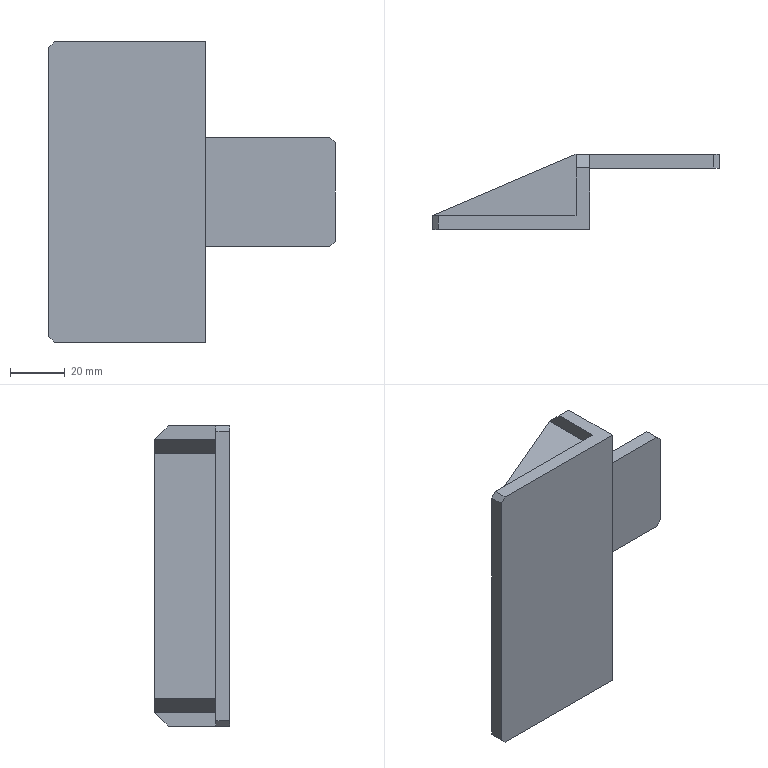Part | STEP file | Guide wheel mechanism revised.sldasm-Part-403 | 1 solid | 28 faces | box 105 x 27.5 x 110 mm | volume 59241 mm3 | plane 28
STEP:
#1=CARTESIAN_POINT('',(0.,22.5,45.));
#2=VERTEX_POINT('',#1);
#3=CARTESIAN_POINT('',(0.,22.5,-45.));
#4=VERTEX_POINT('',#3);
#5=CARTESIAN_POINT('',(0.,22.5,55.));
#6=DIRECTION('',(0.,0.,-1.));
#7=VECTOR('',#6,1000.);
#8=LINE('',#5,#7);
#9=EDGE_CURVE('',#2,#4,#8,.T.);
#10=ORIENTED_EDGE('',*,*,#9,.T.);
#11=CARTESIAN_POINT('',(0.,0.,-45.));
#12=VERTEX_POINT('',#11);
#13=CARTESIAN_POINT('',(0.,22.5,-45.));
#14=DIRECTION('',(0.,-1.,0.));
#15=VECTOR('',#14,1000.);
#16=LINE('',#13,#15);
#17=EDGE_CURVE('',#4,#12,#16,.T.);
#18=ORIENTED_EDGE('',*,*,#17,.T.);
#19=CARTESIAN_POINT('',(0.,0.,45.));
#20=VERTEX_POINT('',#19);
#21=CARTESIAN_POINT('',(0.,0.,55.));
#22=DIRECTION('',(0.,0.,-1.));
#23=VECTOR('',#22,1000.);
#24=LINE('',#21,#23);
#25=EDGE_CURVE('',#20,#12,#24,.T.);
#26=ORIENTED_EDGE('',*,*,#25,.F.);
#27=CARTESIAN_POINT('',(0.,22.5,45.));
#28=DIRECTION('',(0.,1.,0.));
#29=VECTOR('',#28,1000.);
#30=LINE('',#27,#29);
#31=EDGE_CURVE('',#20,#2,#30,.T.);
#32=ORIENTED_EDGE('',*,*,#31,.T.);
#33=EDGE_LOOP('',(#10,#18,#26,#32));
#34=FACE_OUTER_BOUND('',#33,.T.);
#35=CARTESIAN_POINT('',(0.,0.,55.));
#36=DIRECTION('',(-1.,0.,0.));
#37=DIRECTION('',(0.,0.,1.));
#38=AXIS2_PLACEMENT_3D('',#35,#36,#37);
#39=PLANE('',#38);
#40=ADVANCED_FACE('',(#34),#39,.T.);
#41=ORIENTED_EDGE('',*,*,#25,.T.);
#42=CARTESIAN_POINT('',(-52.5,0.,-45.));
#43=VERTEX_POINT('',#42);
#44=CARTESIAN_POINT('',(0.,0.,-45.));
#45=DIRECTION('',(-1.,0.,0.));
#46=VECTOR('',#45,1000.);
#47=LINE('',#44,#46);
#48=EDGE_CURVE('',#12,#43,#47,.T.);
#49=ORIENTED_EDGE('',*,*,#48,.T.);
#50=CARTESIAN_POINT('',(-52.5,0.,45.));
#51=VERTEX_POINT('',#50);
#52=CARTESIAN_POINT('',(-52.5,0.,55.));
#53=DIRECTION('',(0.,0.,-1.));
#54=VECTOR('',#53,1000.);
#55=LINE('',#52,#54);
#56=EDGE_CURVE('',#51,#43,#55,.T.);
#57=ORIENTED_EDGE('',*,*,#56,.F.);
#58=CARTESIAN_POINT('',(0.,0.,45.));
#59=DIRECTION('',(1.,0.,0.));
#60=VECTOR('',#59,1000.);
#61=LINE('',#58,#60);
#62=EDGE_CURVE('',#51,#20,#61,.T.);
#63=ORIENTED_EDGE('',*,*,#62,.T.);
#64=EDGE_LOOP('',(#41,#49,#57,#63));
#65=FACE_OUTER_BOUND('',#64,.T.);
#66=CARTESIAN_POINT('',(0.,0.,55.));
#67=DIRECTION('',(0.,1.,0.));
#68=DIRECTION('',(0.,0.,1.));
#69=AXIS2_PLACEMENT_3D('',#66,#67,#68);
#70=PLANE('',#69);
#71=ADVANCED_FACE('',(#65),#70,.T.);
#72=CARTESIAN_POINT('',(0.,22.5,-50.));
#73=VERTEX_POINT('',#72);
#74=CARTESIAN_POINT('',(0.,0.,-50.));
#75=VERTEX_POINT('',#74);
#76=CARTESIAN_POINT('',(0.,22.5,-50.));
#77=DIRECTION('',(0.,-1.,0.));
#78=VECTOR('',#77,1000.);
#79=LINE('',#76,#78);
#80=EDGE_CURVE('',#73,#75,#79,.T.);
#81=ORIENTED_EDGE('',*,*,#80,.F.);
#82=CARTESIAN_POINT('',(0.,17.5,-55.));
#83=VERTEX_POINT('',#82);
#84=CARTESIAN_POINT('',(0.,63.75,-8.75));
#85=DIRECTION('',(0.,-0.7071,-0.7071));
#86=VECTOR('',#85,1000.);
#87=LINE('',#84,#86);
#88=EDGE_CURVE('',#73,#83,#87,.T.);
#89=ORIENTED_EDGE('',*,*,#88,.T.);
#90=CARTESIAN_POINT('',(0.,0.,-55.));
#91=VERTEX_POINT('',#90);
#92=CARTESIAN_POINT('',(0.,0.,-55.));
#93=DIRECTION('',(0.,1.,0.));
#94=VECTOR('',#93,1000.);
#95=LINE('',#92,#94);
#96=EDGE_CURVE('',#91,#83,#95,.T.);
#97=ORIENTED_EDGE('',*,*,#96,.F.);
#98=CARTESIAN_POINT('',(0.,0.,55.));
#99=DIRECTION('',(0.,0.,-1.));
#100=VECTOR('',#99,1000.);
#101=LINE('',#98,#100);
#102=EDGE_CURVE('',#75,#91,#101,.T.);
#103=ORIENTED_EDGE('',*,*,#102,.F.);
#104=EDGE_LOOP('',(#81,#89,#97,#103));
#105=FACE_OUTER_BOUND('',#104,.T.);
#106=CARTESIAN_POINT('',(0.,0.,55.));
#107=DIRECTION('',(-1.,0.,0.));
#108=DIRECTION('',(0.,0.,1.));
#109=AXIS2_PLACEMENT_3D('',#106,#107,#108);
#110=PLANE('',#109);
#111=ADVANCED_FACE('',(#105),#110,.T.);
#112=CARTESIAN_POINT('',(-52.5,0.,-50.));
#113=VERTEX_POINT('',#112);
#114=CARTESIAN_POINT('',(0.,0.,-50.));
#115=DIRECTION('',(-1.,0.,0.));
#116=VECTOR('',#115,1000.);
#117=LINE('',#114,#116);
#118=EDGE_CURVE('',#75,#113,#117,.T.);
#119=ORIENTED_EDGE('',*,*,#118,.F.);
#120=ORIENTED_EDGE('',*,*,#102,.T.);
#121=CARTESIAN_POINT('',(-50.5,0.,-55.));
#122=VERTEX_POINT('',#121);
#123=CARTESIAN_POINT('',(0.,0.,-55.));
#124=DIRECTION('',(1.,0.,0.));
#125=VECTOR('',#124,1000.);
#126=LINE('',#123,#125);
#127=EDGE_CURVE('',#122,#91,#126,.T.);
#128=ORIENTED_EDGE('',*,*,#127,.F.);
#129=CARTESIAN_POINT('',(-52.5,0.,-53.));
#130=VERTEX_POINT('',#129);
#131=CARTESIAN_POINT('',(-80.25,0.,-25.25));
#132=DIRECTION('',(-0.7071,0.,0.7071));
#133=VECTOR('',#132,1000.);
#134=LINE('',#131,#133);
#135=EDGE_CURVE('',#122,#130,#134,.T.);
#136=ORIENTED_EDGE('',*,*,#135,.T.);
#137=CARTESIAN_POINT('',(-52.5,0.,55.));
#138=DIRECTION('',(0.,0.,-1.));
#139=VECTOR('',#138,1000.);
#140=LINE('',#137,#139);
#141=EDGE_CURVE('',#113,#130,#140,.T.);
#142=ORIENTED_EDGE('',*,*,#141,.F.);
#143=EDGE_LOOP('',(#119,#120,#128,#136,#142));
#144=FACE_OUTER_BOUND('',#143,.T.);
#145=CARTESIAN_POINT('',(0.,0.,55.));
#146=DIRECTION('',(0.,1.,0.));
#147=DIRECTION('',(0.,0.,1.));
#148=AXIS2_PLACEMENT_3D('',#145,#146,#147);
#149=PLANE('',#148);
#150=ADVANCED_FACE('',(#144),#149,.T.);
#151=CARTESIAN_POINT('',(50.5,17.5,-20.));
#152=VERTEX_POINT('',#151);
#153=CARTESIAN_POINT('',(5.,17.5,-20.));
#154=VERTEX_POINT('',#153);
#155=CARTESIAN_POINT('',(52.5,17.5,-20.));
#156=DIRECTION('',(-1.,0.,0.));
#157=VECTOR('',#156,1000.);
#158=LINE('',#155,#157);
#159=EDGE_CURVE('',#152,#154,#158,.T.);
#160=ORIENTED_EDGE('',*,*,#159,.F.);
#161=CARTESIAN_POINT('',(52.5,17.5,-18.));
#162=VERTEX_POINT('',#161);
#163=CARTESIAN_POINT('',(52.5,17.5,-18.));
#164=DIRECTION('',(0.7071,0.,0.7071));
#165=VECTOR('',#164,1000.);
#166=LINE('',#163,#165);
#167=EDGE_CURVE('',#152,#162,#166,.T.);
#168=ORIENTED_EDGE('',*,*,#167,.T.);
#169=CARTESIAN_POINT('',(52.5,17.5,18.));
#170=VERTEX_POINT('',#169);
#171=CARTESIAN_POINT('',(52.5,17.5,55.));
#172=DIRECTION('',(0.,0.,-1.));
#173=VECTOR('',#172,1000.);
#174=LINE('',#171,#173);
#175=EDGE_CURVE('',#170,#162,#174,.T.);
#176=ORIENTED_EDGE('',*,*,#175,.F.);
#177=CARTESIAN_POINT('',(50.5,17.5,20.));
#178=VERTEX_POINT('',#177);
#179=CARTESIAN_POINT('',(50.5,17.5,20.));
#180=DIRECTION('',(-0.7071,0.,0.7071));
#181=VECTOR('',#180,1000.);
#182=LINE('',#179,#181);
#183=EDGE_CURVE('',#170,#178,#182,.T.);
#184=ORIENTED_EDGE('',*,*,#183,.T.);
#185=CARTESIAN_POINT('',(5.,17.5,20.));
#186=VERTEX_POINT('',#185);
#187=CARTESIAN_POINT('',(52.5,17.5,20.));
#188=DIRECTION('',(1.,0.,0.));
#189=VECTOR('',#188,1000.);
#190=LINE('',#187,#189);
#191=EDGE_CURVE('',#186,#178,#190,.T.);
#192=ORIENTED_EDGE('',*,*,#191,.F.);
#193=CARTESIAN_POINT('',(5.,17.5,55.));
#194=DIRECTION('',(0.,0.,-1.));
#195=VECTOR('',#194,1000.);
#196=LINE('',#193,#195);
#197=EDGE_CURVE('',#186,#154,#196,.T.);
#198=ORIENTED_EDGE('',*,*,#197,.T.);
#199=EDGE_LOOP('',(#160,#168,#176,#184,#192,#198));
#200=FACE_OUTER_BOUND('',#199,.T.);
#201=CARTESIAN_POINT('',(0.,17.5,55.));
#202=DIRECTION('',(0.,1.,0.));
#203=DIRECTION('',(0.,0.,1.));
#204=AXIS2_PLACEMENT_3D('',#201,#202,#203);
#205=PLANE('',#204);
#206=ADVANCED_FACE('',(#200),#205,.F.);
#207=ORIENTED_EDGE('',*,*,#175,.T.);
#208=CARTESIAN_POINT('',(52.5,22.5,-18.));
#209=VERTEX_POINT('',#208);
#210=CARTESIAN_POINT('',(52.5,22.5,-18.));
#211=DIRECTION('',(0.,1.,0.));
#212=VECTOR('',#211,1000.);
#213=LINE('',#210,#212);
#214=EDGE_CURVE('',#162,#209,#213,.T.);
#215=ORIENTED_EDGE('',*,*,#214,.T.);
#216=CARTESIAN_POINT('',(52.5,22.5,18.));
#217=VERTEX_POINT('',#216);
#218=CARTESIAN_POINT('',(52.5,22.5,55.));
#219=DIRECTION('',(0.,0.,-1.));
#220=VECTOR('',#219,1000.);
#221=LINE('',#218,#220);
#222=EDGE_CURVE('',#217,#209,#221,.T.);
#223=ORIENTED_EDGE('',*,*,#222,.F.);
#224=CARTESIAN_POINT('',(52.5,17.5,18.));
#225=DIRECTION('',(0.,-1.,0.));
#226=VECTOR('',#225,1000.);
#227=LINE('',#224,#226);
#228=EDGE_CURVE('',#217,#170,#227,.T.);
#229=ORIENTED_EDGE('',*,*,#228,.T.);
#230=EDGE_LOOP('',(#207,#215,#223,#229));
#231=FACE_OUTER_BOUND('',#230,.T.);
#232=CARTESIAN_POINT('',(52.5,22.5,55.));
#233=DIRECTION('',(1.,0.,0.));
#234=DIRECTION('',(0.,0.,-1.));
#235=AXIS2_PLACEMENT_3D('',#232,#233,#234);
#236=PLANE('',#235);
#237=ADVANCED_FACE('',(#231),#236,.T.);
#238=CARTESIAN_POINT('',(5.,22.5,-50.));
#239=VERTEX_POINT('',#238);
#240=CARTESIAN_POINT('',(5.,22.5,-20.));
#241=VERTEX_POINT('',#240);
#242=CARTESIAN_POINT('',(5.,22.5,-55.));
#243=DIRECTION('',(0.,0.,1.));
#244=VECTOR('',#243,1000.);
#245=LINE('',#242,#244);
#246=EDGE_CURVE('',#239,#241,#245,.T.);
#247=ORIENTED_EDGE('',*,*,#246,.F.);
#248=CARTESIAN_POINT('',(0.,22.5,-50.));
#249=DIRECTION('',(-1.,0.,0.));
#250=VECTOR('',#249,1000.);
#251=LINE('',#248,#250);
#252=EDGE_CURVE('',#239,#73,#251,.T.);
#253=ORIENTED_EDGE('',*,*,#252,.T.);
#254=CARTESIAN_POINT('',(0.,22.5,-45.));
#255=DIRECTION('',(0.,0.,-1.));
#256=VECTOR('',#255,1000.);
#257=LINE('',#254,#256);
#258=EDGE_CURVE('',#4,#73,#257,.T.);
#259=ORIENTED_EDGE('',*,*,#258,.F.);
#260=ORIENTED_EDGE('',*,*,#9,.F.);
#261=CARTESIAN_POINT('',(0.,22.5,50.));
#262=VERTEX_POINT('',#261);
#263=CARTESIAN_POINT('',(0.,22.5,55.));
#264=DIRECTION('',(0.,0.,-1.));
#265=VECTOR('',#264,1000.);
#266=LINE('',#263,#265);
#267=EDGE_CURVE('',#262,#2,#266,.T.);
#268=ORIENTED_EDGE('',*,*,#267,.F.);
#269=CARTESIAN_POINT('',(5.,22.5,50.));
#270=VERTEX_POINT('',#269);
#271=CARTESIAN_POINT('',(5.,22.5,50.));
#272=DIRECTION('',(1.,0.,0.));
#273=VECTOR('',#272,1000.);
#274=LINE('',#271,#273);
#275=EDGE_CURVE('',#262,#270,#274,.T.);
#276=ORIENTED_EDGE('',*,*,#275,.T.);
#277=CARTESIAN_POINT('',(5.,22.5,20.));
#278=VERTEX_POINT('',#277);
#279=CARTESIAN_POINT('',(5.,22.5,55.));
#280=DIRECTION('',(0.,0.,1.));
#281=VECTOR('',#280,1000.);
#282=LINE('',#279,#281);
#283=EDGE_CURVE('',#278,#270,#282,.T.);
#284=ORIENTED_EDGE('',*,*,#283,.F.);
#285=CARTESIAN_POINT('',(50.5,22.5,20.));
#286=VERTEX_POINT('',#285);
#287=CARTESIAN_POINT('',(52.5,22.5,20.));
#288=DIRECTION('',(-1.,0.,0.));
#289=VECTOR('',#288,1000.);
#290=LINE('',#287,#289);
#291=EDGE_CURVE('',#286,#278,#290,.T.);
#292=ORIENTED_EDGE('',*,*,#291,.F.);
#293=CARTESIAN_POINT('',(7.75,22.5,62.75));
#294=DIRECTION('',(0.7071,0.,-0.7071));
#295=VECTOR('',#294,1000.);
#296=LINE('',#293,#295);
#297=EDGE_CURVE('',#286,#217,#296,.T.);
#298=ORIENTED_EDGE('',*,*,#297,.T.);
#299=ORIENTED_EDGE('',*,*,#222,.T.);
#300=CARTESIAN_POINT('',(50.5,22.5,-20.));
#301=VERTEX_POINT('',#300);
#302=CARTESIAN_POINT('',(62.75,22.5,-7.75));
#303=DIRECTION('',(-0.7071,0.,-0.7071));
#304=VECTOR('',#303,1000.);
#305=LINE('',#302,#304);
#306=EDGE_CURVE('',#209,#301,#305,.T.);
#307=ORIENTED_EDGE('',*,*,#306,.T.);
#308=CARTESIAN_POINT('',(52.5,22.5,-20.));
#309=DIRECTION('',(1.,0.,0.));
#310=VECTOR('',#309,1000.);
#311=LINE('',#308,#310);
#312=EDGE_CURVE('',#241,#301,#311,.T.);
#313=ORIENTED_EDGE('',*,*,#312,.F.);
#314=EDGE_LOOP('',(#247,#253,#259,#260,#268,#276,#284,#292,#298,#299,#307,#313));
#315=FACE_OUTER_BOUND('',#314,.T.);
#316=CARTESIAN_POINT('',(0.,22.5,55.));
#317=DIRECTION('',(0.,1.,0.));
#318=DIRECTION('',(0.,0.,1.));
#319=AXIS2_PLACEMENT_3D('',#316,#317,#318);
#320=PLANE('',#319);
#321=ADVANCED_FACE('',(#315),#320,.T.);
#322=CARTESIAN_POINT('',(0.,0.,50.));
#323=VERTEX_POINT('',#322);
#324=CARTESIAN_POINT('',(0.,22.5,50.));
#325=DIRECTION('',(0.,1.,0.));
#326=VECTOR('',#325,1000.);
#327=LINE('',#324,#326);
#328=EDGE_CURVE('',#323,#262,#327,.T.);
#329=ORIENTED_EDGE('',*,*,#328,.F.);
#330=CARTESIAN_POINT('',(0.,0.,55.));
#331=VERTEX_POINT('',#330);
#332=CARTESIAN_POINT('',(0.,0.,55.));
#333=DIRECTION('',(0.,0.,-1.));
#334=VECTOR('',#333,1000.);
#335=LINE('',#332,#334);
#336=EDGE_CURVE('',#331,#323,#335,.T.);
#337=ORIENTED_EDGE('',*,*,#336,.F.);
#338=CARTESIAN_POINT('',(0.,17.5,55.));
#339=VERTEX_POINT('',#338);
#340=CARTESIAN_POINT('',(0.,0.,55.));
#341=DIRECTION('',(0.,1.,0.));
#342=VECTOR('',#341,1000.);
#343=LINE('',#340,#342);
#344=EDGE_CURVE('',#331,#339,#343,.T.);
#345=ORIENTED_EDGE('',*,*,#344,.T.);
#346=CARTESIAN_POINT('',(0.,8.75,63.75));
#347=DIRECTION('',(0.,0.7071,-0.7071));
#348=VECTOR('',#347,1000.);
#349=LINE('',#346,#348);
#350=EDGE_CURVE('',#339,#262,#349,.T.);
#351=ORIENTED_EDGE('',*,*,#350,.T.);
#352=EDGE_LOOP('',(#329,#337,#345,#351));
#353=FACE_OUTER_BOUND('',#352,.T.);
#354=CARTESIAN_POINT('',(0.,0.,55.));
#355=DIRECTION('',(-1.,0.,0.));
#356=DIRECTION('',(0.,0.,1.));
#357=AXIS2_PLACEMENT_3D('',#354,#355,#356);
#358=PLANE('',#357);
#359=ADVANCED_FACE('',(#353),#358,.T.);
#360=CARTESIAN_POINT('',(-52.5,0.,50.));
#361=VERTEX_POINT('',#360);
#362=CARTESIAN_POINT('',(0.,0.,50.));
#363=DIRECTION('',(1.,0.,0.));
#364=VECTOR('',#363,1000.);
#365=LINE('',#362,#364);
#366=EDGE_CURVE('',#361,#323,#365,.T.);
#367=ORIENTED_EDGE('',*,*,#366,.F.);
#368=CARTESIAN_POINT('',(-52.5,0.,53.));
#369=VERTEX_POINT('',#368);
#370=CARTESIAN_POINT('',(-52.5,0.,55.));
#371=DIRECTION('',(0.,0.,-1.));
#372=VECTOR('',#371,1000.);
#373=LINE('',#370,#372);
#374=EDGE_CURVE('',#369,#361,#373,.T.);
#375=ORIENTED_EDGE('',*,*,#374,.F.);
#376=CARTESIAN_POINT('',(-50.5,0.,55.));
#377=VERTEX_POINT('',#376);
#378=CARTESIAN_POINT('',(-25.25,0.,80.25));
#379=DIRECTION('',(0.7071,0.,0.7071));
#380=VECTOR('',#379,1000.);
#381=LINE('',#378,#380);
#382=EDGE_CURVE('',#369,#377,#381,.T.);
#383=ORIENTED_EDGE('',*,*,#382,.T.);
#384=CARTESIAN_POINT('',(0.,0.,55.));
#385=DIRECTION('',(1.,0.,0.));
#386=VECTOR('',#385,1000.);
#387=LINE('',#384,#386);
#388=EDGE_CURVE('',#377,#331,#387,.T.);
#389=ORIENTED_EDGE('',*,*,#388,.T.);
#390=ORIENTED_EDGE('',*,*,#336,.T.);
#391=EDGE_LOOP('',(#367,#375,#383,#389,#390));
#392=FACE_OUTER_BOUND('',#391,.T.);
#393=CARTESIAN_POINT('',(0.,0.,55.));
#394=DIRECTION('',(0.,1.,0.));
#395=DIRECTION('',(0.,0.,1.));
#396=AXIS2_PLACEMENT_3D('',#393,#394,#395);
#397=PLANE('',#396);
#398=ADVANCED_FACE('',(#392),#397,.T.);
#399=CARTESIAN_POINT('',(-52.5,-5.,53.));
#400=VERTEX_POINT('',#399);
#401=CARTESIAN_POINT('',(-52.5,-5.,-53.));
#402=VERTEX_POINT('',#401);
#403=CARTESIAN_POINT('',(-52.5,-5.,55.));
#404=DIRECTION('',(0.,0.,-1.));
#405=VECTOR('',#404,1000.);
#406=LINE('',#403,#405);
#407=EDGE_CURVE('',#400,#402,#406,.T.);
#408=ORIENTED_EDGE('',*,*,#407,.F.);
#409=CARTESIAN_POINT('',(-52.5,0.,53.));
#410=DIRECTION('',(0.,1.,0.));
#411=VECTOR('',#410,1000.);
#412=LINE('',#409,#411);
#413=EDGE_CURVE('',#400,#369,#412,.T.);
#414=ORIENTED_EDGE('',*,*,#413,.T.);
#415=ORIENTED_EDGE('',*,*,#374,.T.);
#416=CARTESIAN_POINT('',(-52.5,0.,45.));
#417=DIRECTION('',(0.,0.,1.));
#418=VECTOR('',#417,1000.);
#419=LINE('',#416,#418);
#420=EDGE_CURVE('',#51,#361,#419,.T.);
#421=ORIENTED_EDGE('',*,*,#420,.F.);
#422=ORIENTED_EDGE('',*,*,#56,.T.);
#423=CARTESIAN_POINT('',(-52.5,0.,-45.));
#424=DIRECTION('',(0.,0.,-1.));
#425=VECTOR('',#424,1000.);
#426=LINE('',#423,#425);
#427=EDGE_CURVE('',#43,#113,#426,.T.);
#428=ORIENTED_EDGE('',*,*,#427,.T.);
#429=ORIENTED_EDGE('',*,*,#141,.T.);
#430=CARTESIAN_POINT('',(-52.5,-5.,-53.));
#431=DIRECTION('',(0.,-1.,0.));
#432=VECTOR('',#431,1000.);
#433=LINE('',#430,#432);
#434=EDGE_CURVE('',#130,#402,#433,.T.);
#435=ORIENTED_EDGE('',*,*,#434,.T.);
#436=EDGE_LOOP('',(#408,#414,#415,#421,#422,#428,#429,#435));
#437=FACE_OUTER_BOUND('',#436,.T.);
#438=CARTESIAN_POINT('',(-52.5,-5.,55.));
#439=DIRECTION('',(-1.,0.,0.));
#440=DIRECTION('',(0.,0.,1.));
#441=AXIS2_PLACEMENT_3D('',#438,#439,#440);
#442=PLANE('',#441);
#443=ADVANCED_FACE('',(#437),#442,.T.);
#444=CARTESIAN_POINT('',(-50.5,-5.,55.));
#445=VERTEX_POINT('',#444);
#446=CARTESIAN_POINT('',(5.,-5.,55.));
#447=VERTEX_POINT('',#446);
#448=CARTESIAN_POINT('',(0.,-5.,55.));
#449=DIRECTION('',(1.,0.,0.));
#450=VECTOR('',#449,1000.);
#451=LINE('',#448,#450);
#452=EDGE_CURVE('',#445,#447,#451,.T.);
#453=ORIENTED_EDGE('',*,*,#452,.F.);
#454=CARTESIAN_POINT('',(-52.5,-5.,53.));
#455=DIRECTION('',(-0.7071,0.,-0.7071));
#456=VECTOR('',#455,1000.);
#457=LINE('',#454,#456);
#458=EDGE_CURVE('',#445,#400,#457,.T.);
#459=ORIENTED_EDGE('',*,*,#458,.T.);
#460=ORIENTED_EDGE('',*,*,#407,.T.);
#461=CARTESIAN_POINT('',(-50.5,-5.,-55.));
#462=VERTEX_POINT('',#461);
#463=CARTESIAN_POINT('',(-50.5,-5.,-55.));
#464=DIRECTION('',(0.7071,0.,-0.7071));
#465=VECTOR('',#464,1000.);
#466=LINE('',#463,#465);
#467=EDGE_CURVE('',#402,#462,#466,.T.);
#468=ORIENTED_EDGE('',*,*,#467,.T.);
#469=CARTESIAN_POINT('',(5.,-5.,-55.));
#470=VERTEX_POINT('',#469);
#471=CARTESIAN_POINT('',(0.,-5.,-55.));
#472=DIRECTION('',(1.,0.,0.));
#473=VECTOR('',#472,1000.);
#474=LINE('',#471,#473);
#475=EDGE_CURVE('',#462,#470,#474,.T.);
#476=ORIENTED_EDGE('',*,*,#475,.T.);
#477=CARTESIAN_POINT('',(5.,-5.,55.));
#478=DIRECTION('',(0.,0.,-1.));
#479=VECTOR('',#478,1000.);
#480=LINE('',#477,#479);
#481=EDGE_CURVE('',#447,#470,#480,.T.);
#482=ORIENTED_EDGE('',*,*,#481,.F.);
#483=EDGE_LOOP('',(#453,#459,#460,#468,#476,#482));
#484=FACE_OUTER_BOUND('',#483,.T.);
#485=CARTESIAN_POINT('',(0.,-5.,55.));
#486=DIRECTION('',(0.,1.,0.));
#487=DIRECTION('',(0.,0.,1.));
#488=AXIS2_PLACEMENT_3D('',#485,#486,#487);
#489=PLANE('',#488);
#490=ADVANCED_FACE('',(#484),#489,.F.);
#491=CARTESIAN_POINT('',(5.,17.5,-55.));
#492=VERTEX_POINT('',#491);
#493=CARTESIAN_POINT('',(5.,0.,-55.));
#494=DIRECTION('',(0.,1.,0.));
#495=VECTOR('',#494,1000.);
#496=LINE('',#493,#495);
#497=EDGE_CURVE('',#470,#492,#496,.T.);
#498=ORIENTED_EDGE('',*,*,#497,.T.);
#499=CARTESIAN_POINT('',(5.,17.5,-55.));
#500=DIRECTION('',(0.,0.7071,0.7071));
#501=VECTOR('',#500,1000.);
#502=LINE('',#499,#501);
#503=EDGE_CURVE('',#492,#239,#502,.T.);
#504=ORIENTED_EDGE('',*,*,#503,.T.);
#505=ORIENTED_EDGE('',*,*,#246,.T.);
#506=CARTESIAN_POINT('',(5.,-5.001,-20.));
#507=DIRECTION('',(0.,1.,0.));
#508=VECTOR('',#507,1000.);
#509=LINE('',#506,#508);
#510=EDGE_CURVE('',#154,#241,#509,.T.);
#511=ORIENTED_EDGE('',*,*,#510,.F.);
#512=ORIENTED_EDGE('',*,*,#197,.F.);
#513=CARTESIAN_POINT('',(5.,-5.001,20.));
#514=DIRECTION('',(0.,1.,0.));
#515=VECTOR('',#514,1000.);
#516=LINE('',#513,#515);
#517=EDGE_CURVE('',#186,#278,#516,.T.);
#518=ORIENTED_EDGE('',*,*,#517,.T.);
#519=ORIENTED_EDGE('',*,*,#283,.T.);
#520=CARTESIAN_POINT('',(5.,17.5,55.));
#521=VERTEX_POINT('',#520);
#522=CARTESIAN_POINT('',(5.,22.5,50.));
#523=DIRECTION('',(0.,-0.7071,0.7071));
#524=VECTOR('',#523,1000.);
#525=LINE('',#522,#524);
#526=EDGE_CURVE('',#270,#521,#525,.T.);
#527=ORIENTED_EDGE('',*,*,#526,.T.);
#528=CARTESIAN_POINT('',(5.,0.,55.));
#529=DIRECTION('',(0.,1.,0.));
#530=VECTOR('',#529,1000.);
#531=LINE('',#528,#530);
#532=EDGE_CURVE('',#447,#521,#531,.T.);
#533=ORIENTED_EDGE('',*,*,#532,.F.);
#534=ORIENTED_EDGE('',*,*,#481,.T.);
#535=EDGE_LOOP('',(#498,#504,#505,#511,#512,#518,#519,#527,#533,#534));
#536=FACE_OUTER_BOUND('',#535,.T.);
#537=CARTESIAN_POINT('',(5.,0.,55.));
#538=DIRECTION('',(-1.,0.,0.));
#539=DIRECTION('',(0.,0.,1.));
#540=AXIS2_PLACEMENT_3D('',#537,#538,#539);
#541=PLANE('',#540);
#542=ADVANCED_FACE('',(#536),#541,.F.);
#543=ORIENTED_EDGE('',*,*,#532,.T.);
#544=CARTESIAN_POINT('',(0.,17.5,55.));
#545=DIRECTION('',(-1.,0.,0.));
#546=VECTOR('',#545,1000.);
#547=LINE('',#544,#546);
#548=EDGE_CURVE('',#521,#339,#547,.T.);
#549=ORIENTED_EDGE('',*,*,#548,.T.);
#550=ORIENTED_EDGE('',*,*,#344,.F.);
#551=ORIENTED_EDGE('',*,*,#388,.F.);
#552=CARTESIAN_POINT('',(-50.5,-5.,55.));
#553=DIRECTION('',(0.,-1.,0.));
#554=VECTOR('',#553,1000.);
#555=LINE('',#552,#554);
#556=EDGE_CURVE('',#377,#445,#555,.T.);
#557=ORIENTED_EDGE('',*,*,#556,.T.);
#558=ORIENTED_EDGE('',*,*,#452,.T.);
#559=EDGE_LOOP('',(#543,#549,#550,#551,#557,#558));
#560=FACE_OUTER_BOUND('',#559,.T.);
#561=CARTESIAN_POINT('',(0.,0.,55.));
#562=DIRECTION('',(0.,0.,-1.));
#563=DIRECTION('',(-1.,0.,0.));
#564=AXIS2_PLACEMENT_3D('',#561,#562,#563);
#565=PLANE('',#564);
#566=ADVANCED_FACE('',(#560),#565,.F.);
#567=ORIENTED_EDGE('',*,*,#96,.T.);
#568=CARTESIAN_POINT('',(0.,17.5,-55.));
#569=DIRECTION('',(1.,0.,0.));
#570=VECTOR('',#569,1000.);
#571=LINE('',#568,#570);
#572=EDGE_CURVE('',#83,#492,#571,.T.);
#573=ORIENTED_EDGE('',*,*,#572,.T.);
#574=ORIENTED_EDGE('',*,*,#497,.F.);
#575=ORIENTED_EDGE('',*,*,#475,.F.);
#576=CARTESIAN_POINT('',(-50.5,0.,-55.));
#577=DIRECTION('',(0.,1.,0.));
#578=VECTOR('',#577,1000.);
#579=LINE('',#576,#578);
#580=EDGE_CURVE('',#462,#122,#579,.T.);
#581=ORIENTED_EDGE('',*,*,#580,.T.);
#582=ORIENTED_EDGE('',*,*,#127,.T.);
#583=EDGE_LOOP('',(#567,#573,#574,#575,#581,#582));
#584=FACE_OUTER_BOUND('',#583,.T.);
#585=CARTESIAN_POINT('',(0.,0.,-55.));
#586=DIRECTION('',(0.,0.,-1.));
#587=DIRECTION('',(-1.,0.,0.));
#588=AXIS2_PLACEMENT_3D('',#585,#586,#587);
#589=PLANE('',#588);
#590=ADVANCED_FACE('',(#584),#589,.T.);
#591=ORIENTED_EDGE('',*,*,#312,.T.);
#592=CARTESIAN_POINT('',(50.5,17.5,-20.));
#593=DIRECTION('',(0.,-1.,0.));
#594=VECTOR('',#593,1000.);
#595=LINE('',#592,#594);
#596=EDGE_CURVE('',#301,#152,#595,.T.);
#597=ORIENTED_EDGE('',*,*,#596,.T.);
#598=ORIENTED_EDGE('',*,*,#159,.T.);
#599=ORIENTED_EDGE('',*,*,#510,.T.);
#600=EDGE_LOOP('',(#591,#597,#598,#599));
#601=FACE_OUTER_BOUND('',#600,.T.);
#602=CARTESIAN_POINT('',(52.5,-5.001,-20.));
#603=DIRECTION('',(0.,0.,1.));
#604=DIRECTION('',(1.,0.,0.));
#605=AXIS2_PLACEMENT_3D('',#602,#603,#604);
#606=PLANE('',#605);
#607=ADVANCED_FACE('',(#601),#606,.F.);
#608=ORIENTED_EDGE('',*,*,#191,.T.);
#609=CARTESIAN_POINT('',(50.5,22.5,20.));
#610=DIRECTION('',(0.,1.,0.));
#611=VECTOR('',#610,1000.);
#612=LINE('',#609,#611);
#613=EDGE_CURVE('',#178,#286,#612,.T.);
#614=ORIENTED_EDGE('',*,*,#613,.T.);
#615=ORIENTED_EDGE('',*,*,#291,.T.);
#616=ORIENTED_EDGE('',*,*,#517,.F.);
#617=EDGE_LOOP('',(#608,#614,#615,#616));
#618=FACE_OUTER_BOUND('',#617,.T.);
#619=CARTESIAN_POINT('',(52.5,-5.001,20.));
#620=DIRECTION('',(0.,0.,-1.));
#621=DIRECTION('',(-1.,0.,0.));
#622=AXIS2_PLACEMENT_3D('',#619,#620,#621);
#623=PLANE('',#622);
#624=ADVANCED_FACE('',(#618),#623,.F.);
#625=ORIENTED_EDGE('',*,*,#458,.F.);
#626=ORIENTED_EDGE('',*,*,#556,.F.);
#627=ORIENTED_EDGE('',*,*,#382,.F.);
#628=ORIENTED_EDGE('',*,*,#413,.F.);
#629=EDGE_LOOP('',(#625,#626,#627,#628));
#630=FACE_OUTER_BOUND('',#629,.T.);
#631=CARTESIAN_POINT('',(-52.5,-5.,53.));
#632=DIRECTION('',(-0.7071,0.,0.7071));
#633=DIRECTION('',(0.,-1.,0.));
#634=AXIS2_PLACEMENT_3D('',#631,#632,#633);
#635=PLANE('',#634);
#636=ADVANCED_FACE('',(#630),#635,.T.);
#637=ORIENTED_EDGE('',*,*,#467,.F.);
#638=ORIENTED_EDGE('',*,*,#434,.F.);
#639=ORIENTED_EDGE('',*,*,#135,.F.);
#640=ORIENTED_EDGE('',*,*,#580,.F.);
#641=EDGE_LOOP('',(#637,#638,#639,#640));
#642=FACE_OUTER_BOUND('',#641,.T.);
#643=CARTESIAN_POINT('',(-50.5,0.,-55.));
#644=DIRECTION('',(0.7071,0.,0.7071));
#645=DIRECTION('',(0.,1.,0.));
#646=AXIS2_PLACEMENT_3D('',#643,#644,#645);
#647=PLANE('',#646);
#648=ADVANCED_FACE('',(#642),#647,.F.);
#649=ORIENTED_EDGE('',*,*,#167,.F.);
#650=ORIENTED_EDGE('',*,*,#596,.F.);
#651=ORIENTED_EDGE('',*,*,#306,.F.);
#652=ORIENTED_EDGE('',*,*,#214,.F.);
#653=EDGE_LOOP('',(#649,#650,#651,#652));
#654=FACE_OUTER_BOUND('',#653,.T.);
#655=CARTESIAN_POINT('',(52.5,22.5,-18.));
#656=DIRECTION('',(0.7071,0.,-0.7071));
#657=DIRECTION('',(0.,-1.,0.));
#658=AXIS2_PLACEMENT_3D('',#655,#656,#657);
#659=PLANE('',#658);
#660=ADVANCED_FACE('',(#654),#659,.T.);
#661=ORIENTED_EDGE('',*,*,#183,.F.);
#662=ORIENTED_EDGE('',*,*,#228,.F.);
#663=ORIENTED_EDGE('',*,*,#297,.F.);
#664=ORIENTED_EDGE('',*,*,#613,.F.);
#665=EDGE_LOOP('',(#661,#662,#663,#664));
#666=FACE_OUTER_BOUND('',#665,.T.);
#667=CARTESIAN_POINT('',(50.5,-5.001,20.));
#668=DIRECTION('',(0.7071,0.,0.7071));
#669=DIRECTION('',(0.,-1.,0.));
#670=AXIS2_PLACEMENT_3D('',#667,#668,#669);
#671=PLANE('',#670);
#672=ADVANCED_FACE('',(#666),#671,.T.);
#673=ORIENTED_EDGE('',*,*,#88,.F.);
#674=ORIENTED_EDGE('',*,*,#252,.F.);
#675=ORIENTED_EDGE('',*,*,#503,.F.);
#676=ORIENTED_EDGE('',*,*,#572,.F.);
#677=EDGE_LOOP('',(#673,#674,#675,#676));
#678=FACE_OUTER_BOUND('',#677,.T.);
#679=CARTESIAN_POINT('',(0.,17.5,-55.));
#680=DIRECTION('',(0.,-0.7071,0.7071));
#681=DIRECTION('',(1.,0.,0.));
#682=AXIS2_PLACEMENT_3D('',#679,#680,#681);
#683=PLANE('',#682);
#684=ADVANCED_FACE('',(#678),#683,.F.);
#685=ORIENTED_EDGE('',*,*,#350,.F.);
#686=ORIENTED_EDGE('',*,*,#548,.F.);
#687=ORIENTED_EDGE('',*,*,#526,.F.);
#688=ORIENTED_EDGE('',*,*,#275,.F.);
#689=EDGE_LOOP('',(#685,#686,#687,#688));
#690=FACE_OUTER_BOUND('',#689,.T.);
#691=CARTESIAN_POINT('',(0.,22.5,50.));
#692=DIRECTION('',(0.,0.7071,0.7071));
#693=DIRECTION('',(-1.,0.,0.));
#694=AXIS2_PLACEMENT_3D('',#691,#692,#693);
#695=PLANE('',#694);
#696=ADVANCED_FACE('',(#690),#695,.T.);
#697=CARTESIAN_POINT('',(-52.5,0.,50.));
#698=DIRECTION('',(-0.9191,-0.3939,0.));
#699=VECTOR('',#698,1000.);
#700=LINE('',#697,#699);
#701=EDGE_CURVE('',#262,#361,#700,.T.);
#702=ORIENTED_EDGE('',*,*,#701,.F.);
#703=ORIENTED_EDGE('',*,*,#267,.T.);
#704=CARTESIAN_POINT('',(-52.5,0.,45.));
#705=DIRECTION('',(-0.9191,-0.3939,0.));
#706=VECTOR('',#705,1000.);
#707=LINE('',#704,#706);
#708=EDGE_CURVE('',#2,#51,#707,.T.);
#709=ORIENTED_EDGE('',*,*,#708,.T.);
#710=ORIENTED_EDGE('',*,*,#420,.T.);
#711=EDGE_LOOP('',(#702,#703,#709,#710));
#712=FACE_OUTER_BOUND('',#711,.T.);
#713=CARTESIAN_POINT('',(-52.5,0.,45.));
#714=DIRECTION('',(-0.3939,0.9191,0.));
#715=DIRECTION('',(-0.9191,-0.3939,0.));
#716=AXIS2_PLACEMENT_3D('',#713,#714,#715);
#717=PLANE('',#716);
#718=ADVANCED_FACE('',(#712),#717,.T.);
#719=ORIENTED_EDGE('',*,*,#62,.F.);
#720=ORIENTED_EDGE('',*,*,#708,.F.);
#721=ORIENTED_EDGE('',*,*,#31,.F.);
#722=EDGE_LOOP('',(#719,#720,#721));
#723=FACE_OUTER_BOUND('',#722,.T.);
#724=CARTESIAN_POINT('',(0.,0.,45.));
#725=DIRECTION('',(0.,0.,1.));
#726=DIRECTION('',(1.,0.,0.));
#727=AXIS2_PLACEMENT_3D('',#724,#725,#726);
#728=PLANE('',#727);
#729=ADVANCED_FACE('',(#723),#728,.F.);
#730=ORIENTED_EDGE('',*,*,#366,.T.);
#731=ORIENTED_EDGE('',*,*,#328,.T.);
#732=ORIENTED_EDGE('',*,*,#701,.T.);
#733=EDGE_LOOP('',(#730,#731,#732));
#734=FACE_OUTER_BOUND('',#733,.T.);
#735=CARTESIAN_POINT('',(0.,0.,50.));
#736=DIRECTION('',(0.,0.,1.));
#737=DIRECTION('',(1.,0.,0.));
#738=AXIS2_PLACEMENT_3D('',#735,#736,#737);
#739=PLANE('',#738);
#740=ADVANCED_FACE('',(#734),#739,.T.);
#741=CARTESIAN_POINT('',(-52.5,0.,-50.));
#742=DIRECTION('',(0.9191,0.3939,0.));
#743=VECTOR('',#742,1000.);
#744=LINE('',#741,#743);
#745=EDGE_CURVE('',#113,#73,#744,.T.);
#746=ORIENTED_EDGE('',*,*,#745,.F.);
#747=ORIENTED_EDGE('',*,*,#427,.F.);
#748=CARTESIAN_POINT('',(-52.5,0.,-45.));
#749=DIRECTION('',(0.9191,0.3939,0.));
#750=VECTOR('',#749,1000.);
#751=LINE('',#748,#750);
#752=EDGE_CURVE('',#43,#4,#751,.T.);
#753=ORIENTED_EDGE('',*,*,#752,.T.);
#754=ORIENTED_EDGE('',*,*,#258,.T.);
#755=EDGE_LOOP('',(#746,#747,#753,#754));
#756=FACE_OUTER_BOUND('',#755,.T.);
#757=CARTESIAN_POINT('',(-52.5,0.,-45.));
#758=DIRECTION('',(-0.3939,0.9191,0.));
#759=DIRECTION('',(-0.9191,-0.3939,0.));
#760=AXIS2_PLACEMENT_3D('',#757,#758,#759);
#761=PLANE('',#760);
#762=ADVANCED_FACE('',(#756),#761,.T.);
#763=ORIENTED_EDGE('',*,*,#752,.F.);
#764=ORIENTED_EDGE('',*,*,#48,.F.);
#765=ORIENTED_EDGE('',*,*,#17,.F.);
#766=EDGE_LOOP('',(#763,#764,#765));
#767=FACE_OUTER_BOUND('',#766,.T.);
#768=CARTESIAN_POINT('',(0.,0.,-45.));
#769=DIRECTION('',(0.,0.,-1.));
#770=DIRECTION('',(-1.,0.,0.));
#771=AXIS2_PLACEMENT_3D('',#768,#769,#770);
#772=PLANE('',#771);
#773=ADVANCED_FACE('',(#767),#772,.F.);
#774=ORIENTED_EDGE('',*,*,#745,.T.);
#775=ORIENTED_EDGE('',*,*,#80,.T.);
#776=ORIENTED_EDGE('',*,*,#118,.T.);
#777=EDGE_LOOP('',(#774,#775,#776));
#778=FACE_OUTER_BOUND('',#777,.T.);
#779=CARTESIAN_POINT('',(0.,0.,-50.));
#780=DIRECTION('',(0.,0.,-1.));
#781=DIRECTION('',(-1.,0.,0.));
#782=AXIS2_PLACEMENT_3D('',#779,#780,#781);
#783=PLANE('',#782);
#784=ADVANCED_FACE('',(#778),#783,.T.);
#785=CLOSED_SHELL('',(#40,#71,#111,#150,#206,#237,#321,#359,#398,#443,#490,#542,#566,#590,#607,#624,#636,#648,#660,#672,#684,#696,#718,#729,#740,#762,#773,#784));
#786=MANIFOLD_SOLID_BREP('',#785);
#787=CARTESIAN_POINT('',(0.,0.,0.));
#788=DIRECTION('',(0.,0.,1.));
#789=DIRECTION('',(1.,0.,0.));
#790=AXIS2_PLACEMENT_3D('',#787,#788,#789);
#791=(LENGTH_UNIT()NAMED_UNIT(*)SI_UNIT(.MILLI.,.METRE.));
#792=UNCERTAINTY_MEASURE_WITH_UNIT(LENGTH_MEASURE(0.00001),#791,'','');
#793=(NAMED_UNIT(*)PLANE_ANGLE_UNIT()SI_UNIT($,.RADIAN.));
#794=(NAMED_UNIT(*)SI_UNIT($,.STERADIAN.)SOLID_ANGLE_UNIT());
#795=(GEOMETRIC_REPRESENTATION_CONTEXT(3)GLOBAL_UNCERTAINTY_ASSIGNED_CONTEXT((#792))GLOBAL_UNIT_ASSIGNED_CONTEXT((#791,#793,#794))REPRESENTATION_CONTEXT('',''));
#796=ADVANCED_BREP_SHAPE_REPRESENTATION('',(#786,#790),#795);